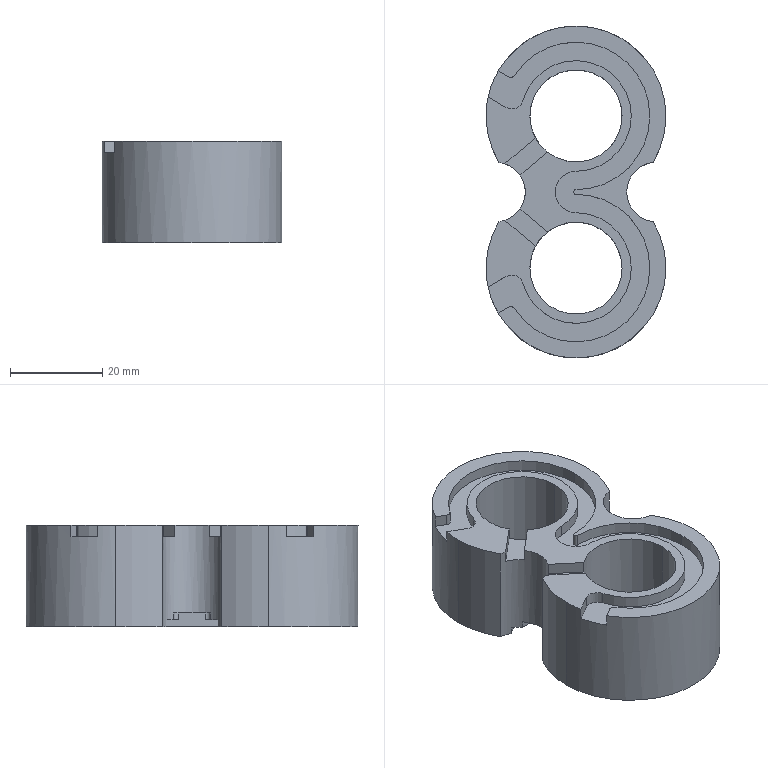Part | SolidWorks | features ICE 4, Extrusion 1, Fillet 1, MirrorPattern 1 | 1 solid | 57 faces | box 39 x 72 x 22 mm | volume 33796 mm3 | cylinder 31 | plane 26 | commonest cylinder face diameters 2 x6 39 x6 20 x4 24 x4 32 x4 13 x3